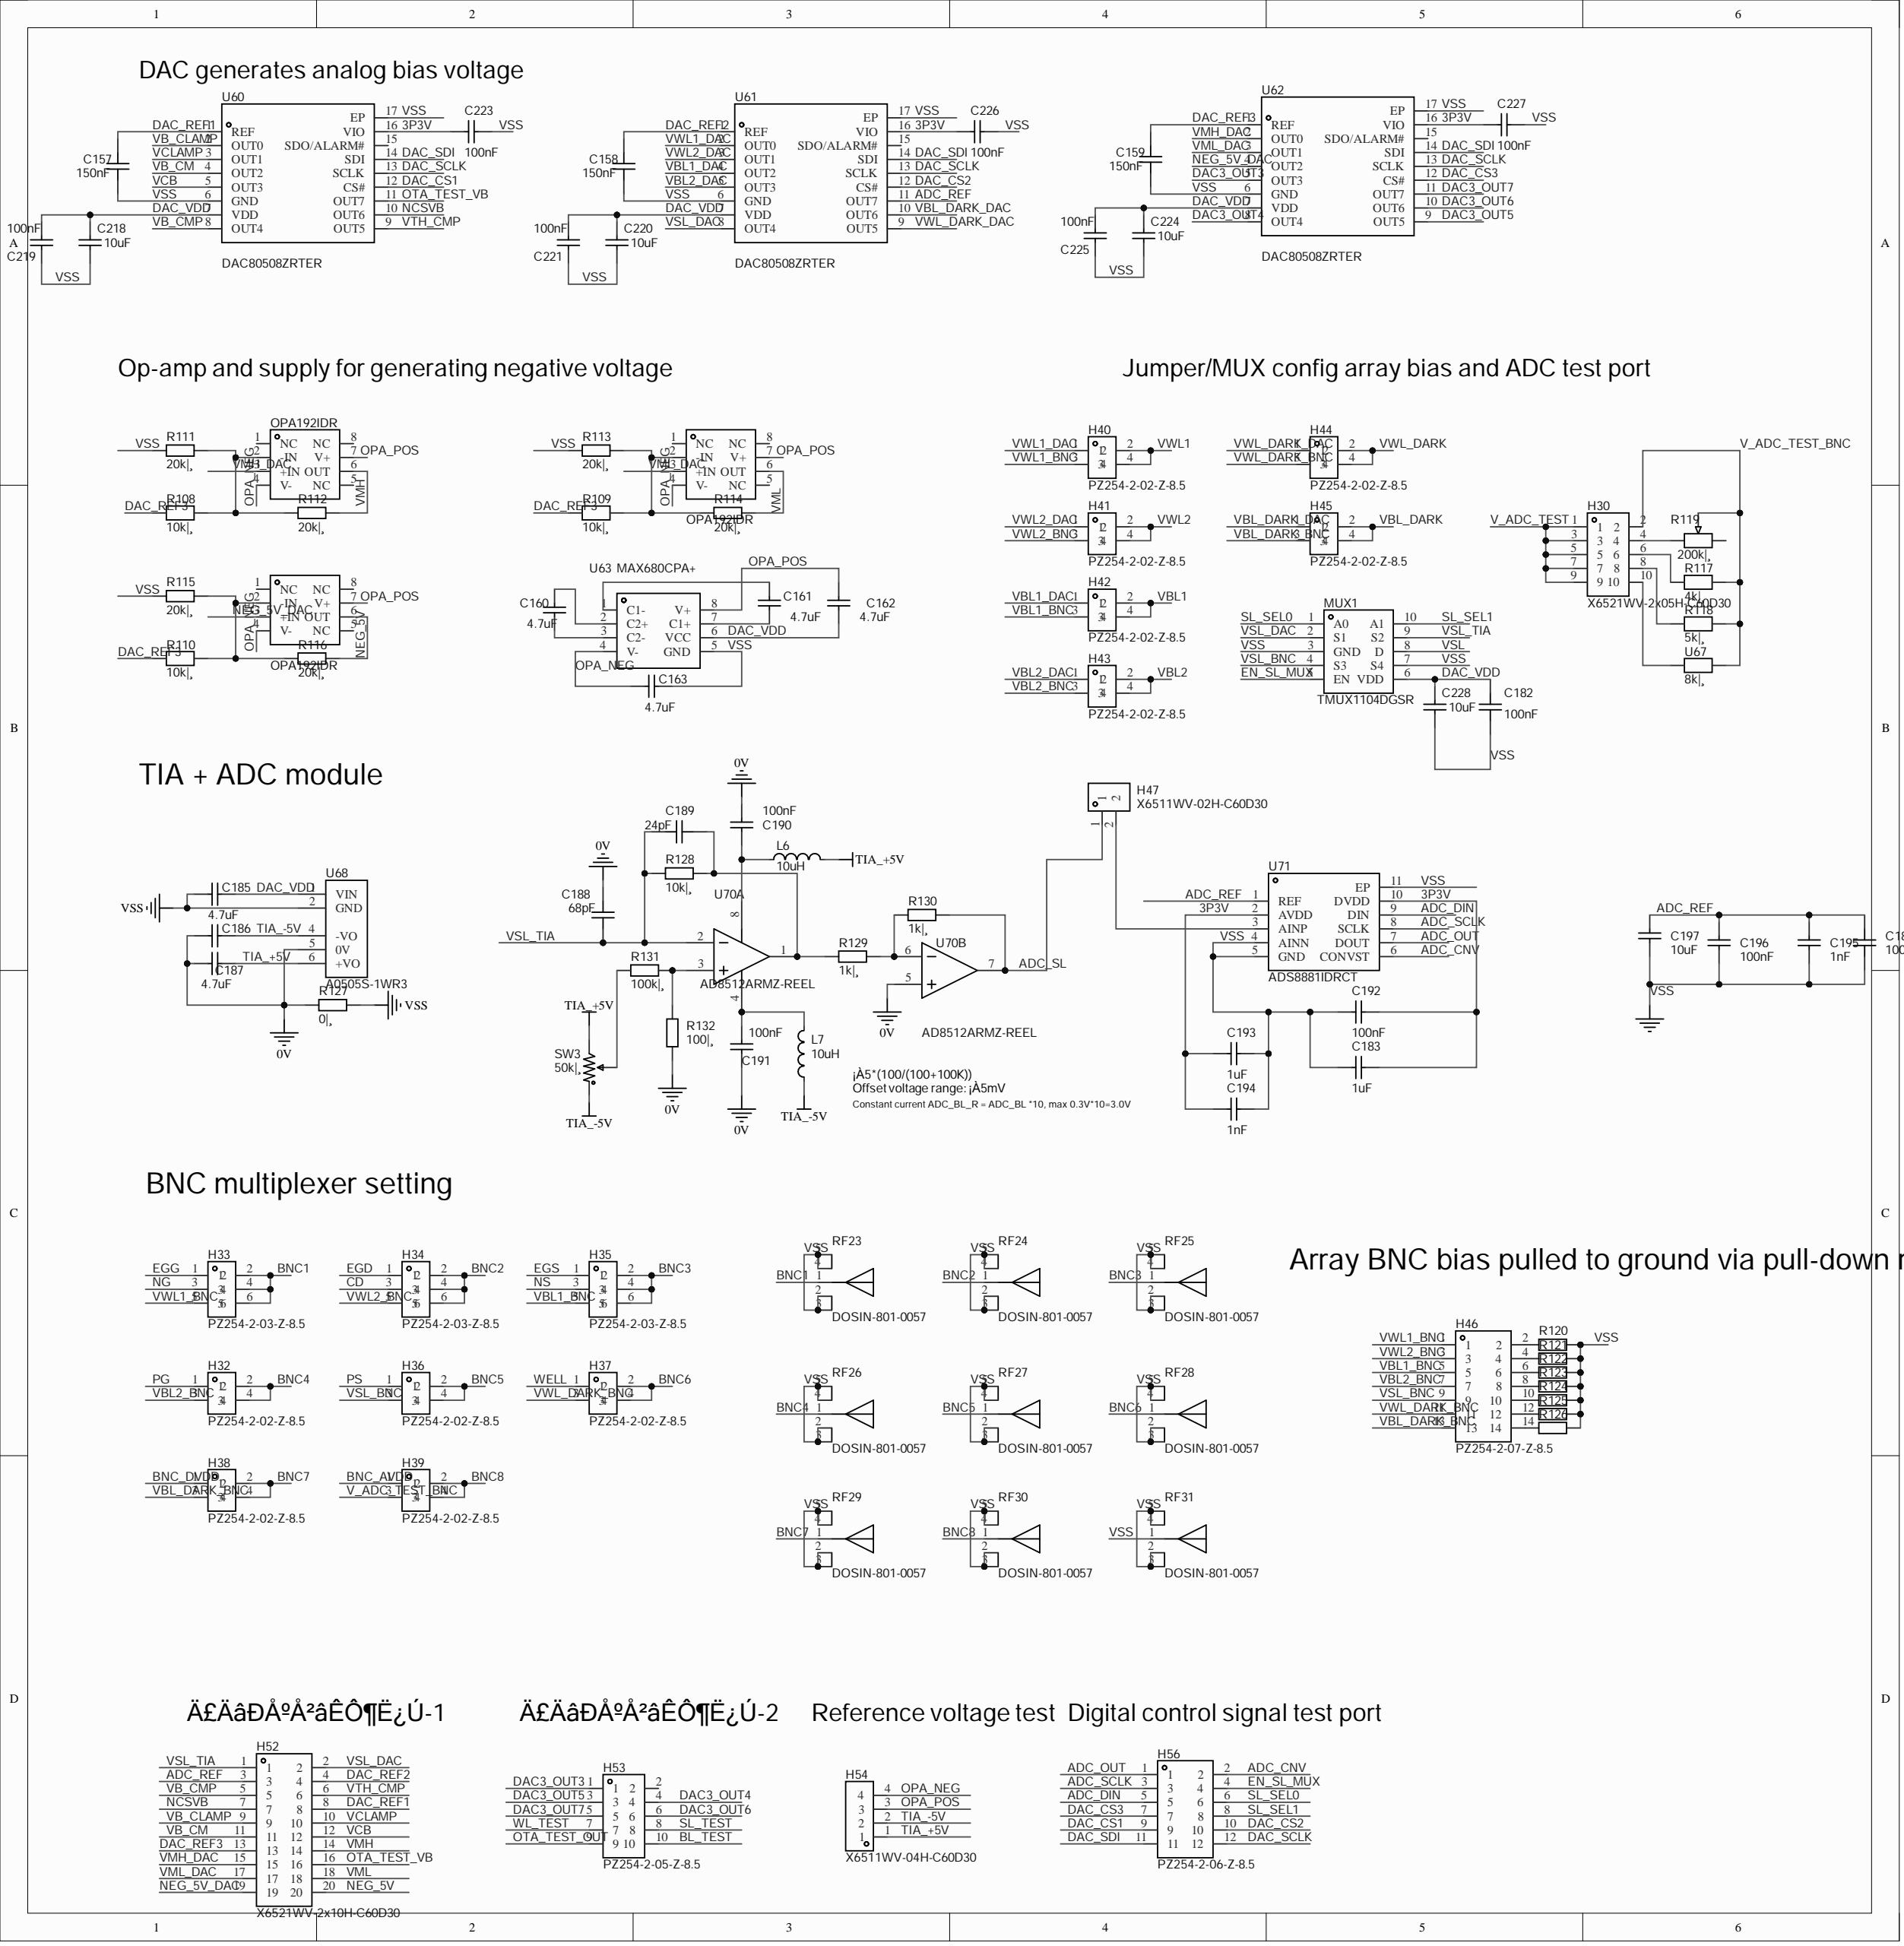Circuit board | Altium Designer | 201 parts | 197 nets | one sheet of the schematic
Parts on this sheet (reference | value | footprint):
C157 | 150nF | C0402
C158 | 150nF | C0402
C159 | 150nF | C0402
C160 | 4.7uF | C0805
C161 | 4.7uF | C0805
C162 | 4.7uF | C0805
C163 | 4.7uF | C0805
C182 | 100nF | C0402
C183 | 1uF | C0603
C184 | 100uF | C1210
C185 | 4.7uF | C0805
C186 | 4.7uF | C0805
C187 | 4.7uF | C0805
C188 | 68pF | C0402
C189 | 24pF | C0402
C190 | 100nF | C0402
C191 | 100nF | C0402
C192 | 100nF | C0402
C193 | 1uF | C0603
C194 | 1nF | C0603
C195 | 1nF | C0603
C196 | 100nF | C0402
C197 | 10uF | C0805
C218 | 10uF | C0805
C219 | 100nF | C0402
C220 | 10uF | C0805
C221 | 100nF | C0402
C223 | 100nF | C0402
C224 | 10uF | C0805
C225 | 100nF | C0402
C226 | 100nF | C0402
C227 | 100nF | C0402
C228 | 10uF | C0805
H30 | X6521WV-2x05H-C60D30 | HDR-TH_10P-P2.54-V-M-R2-C5-S2.54
H32 | PZ254-2-02-Z-8.5 | HDR-TH_4P-P2.54-V-M-R2-C2-S2.54
H33 | PZ254-2-03-Z-8.5 | HDR-TH_6P-P2.54-V-M-R2-C3-S2.54
H34 | PZ254-2-03-Z-8.5 | HDR-TH_6P-P2.54-V-M-R2-C3-S2.54
H35 | PZ254-2-03-Z-8.5 | HDR-TH_6P-P2.54-V-M-R2-C3-S2.54
H36 | PZ254-2-02-Z-8.5 | HDR-TH_4P-P2.54-V-M-R2-C2-S2.54
H37 | PZ254-2-02-Z-8.5 | HDR-TH_4P-P2.54-V-M-R2-C2-S2.54
H38 | PZ254-2-02-Z-8.5 | HDR-TH_4P-P2.54-V-M-R2-C2-S2.54
H39 | PZ254-2-02-Z-8.5 | HDR-TH_4P-P2.54-V-M-R2-C2-S2.54
H40 | PZ254-2-02-Z-8.5 | HDR-TH_4P-P2.54-V-M-R2-C2-S2.54
H41 | PZ254-2-02-Z-8.5 | HDR-TH_4P-P2.54-V-M-R2-C2-S2.54
H42 | PZ254-2-02-Z-8.5 | HDR-TH_4P-P2.54-V-M-R2-C2-S2.54
H43 | PZ254-2-02-Z-8.5 | HDR-TH_4P-P2.54-V-M-R2-C2-S2.54
H44 | PZ254-2-02-Z-8.5 | HDR-TH_4P-P2.54-V-M-R2-C2-S2.54
H45 | PZ254-2-02-Z-8.5 | HDR-TH_4P-P2.54-V-M-R2-C2-S2.54
H46 | PZ254-2-07-Z-8.5 | HDR-TH_14P-P2.54-V-M-R2-C7-S2.54
H47 | X6511WV-02H-C60D30 | HDR-TH_2P-P2.54-V-M
H52 | X6521WV-2x10H-C60D30 | HDR-TH_20P-P2.54-V-M-R2-C10-S2.54
H53 | PZ254-2-05-Z-8.5 | HDR-TH_10P-P2.54-V-M-R2-C5-S2.54
H54 | X6511WV-04H-C60D30 | HDR-TH_4P-P2.54-V-M
H56 | PZ254-2-06-Z-8.5 | HDR-TH_12P-P2.54-V-M-R2-C6-S2.54
L6 | 10uH | IND-SMD_L7.3-W6.8
L7 | 10uH | IND-SMD_L7.3-W6.8
MUX1 | TMUX1104DGSR | VSSOP-10_L3.0-W3.0-P0.50-LS4.9-BL
R108 | 10k|¸ | R0603
R109 | 10k|¸ | R0603
R110 | 10k|¸ | R0603
R111 | 20k|¸ | R0805
R112 | 20k|¸ | R0805
R113 | 20k|¸ | R0805
R114 | 20k|¸ | R0805
R115 | 20k|¸ | R0805
R116 | 20k|¸ | R0805
R117 | 4k|¸ | R0805
R118 | 5k|¸ | R0805
R119 | 200k|¸ | RES-ADJ-SMD_3P-L4.5-W4.5-P2.30-BL-FS
R120 | 1M|¸ | R1206
R121 | 1M|¸ | R1206
R122 | 1M|¸ | R1206
R123 | 1M|¸ | R1206
R124 | 1M|¸ | R1206
R125 | 1M|¸ | R1206
R126 | 1M|¸ | R1206
R127 | 0|¸ | R0603
R128 | 10k|¸ | R0603
R129 | 1k|¸ | R0805
R130 | 1k|¸ | R0805
R131 | 100k|¸ | R0603
R132 | 100|¸ | R1206
RF23 | DOSIN-801-0057 | ANT-TH_DOSIN-801-0057
RF24 | DOSIN-801-0057 | ANT-TH_DOSIN-801-0057
RF25 | DOSIN-801-0057 | ANT-TH_DOSIN-801-0057
RF26 | DOSIN-801-0057 | ANT-TH_DOSIN-801-0057
RF27 | DOSIN-801-0057 | ANT-TH_DOSIN-801-0057
RF28 | DOSIN-801-0057 | ANT-TH_DOSIN-801-0057
RF29 | DOSIN-801-0057 | ANT-TH_DOSIN-801-0057
RF30 | DOSIN-801-0057 | ANT-TH_DOSIN-801-0057
RF31 | DOSIN-801-0057 | ANT-TH_DOSIN-801-0057
SW3 | 50k|¸ | RES-ADJ-SMD_3P-L6.0-W4.3-P5.00-BL
U60 | DAC80508ZRTER | WQFN-16_L3.0-W3.0-P0.50-TL-EP0.8
U61 | DAC80508ZRTER | WQFN-16_L3.0-W3.0-P0.50-TL-EP0.8
U62 | DAC80508ZRTER | WQFN-16_L3.0-W3.0-P0.50-TL-EP0.8
U63 | MAX680CPA+ | DIP-8_L10.1-W6.3-P2.54-LS7.6-BL
U67 | 8k|¸ | R0805
U68 | A0505S-1WR3 | PWRM-TH_A05XXS-1WR3
U71 | ADS8881IDRCT | VSON-10_L3.0-W3.0-P0.50-TL-EP-3
Nets of these parts (net: part-pin ...):
WL_TEST: H53-7
WELL: H37-1
VWL_DARK_DAC: H44-1 U61-9
VWL_DARK_BNC: H37-3 H44-3 H46-11
VWL_DARK: H44-2 H44-4
VWL2_DAC: H41-1 U61-3
VWL2_BNC: H34-5 H41-3 H46-3
VWL2: H41-2 H41-4
VWL1_DAC: H40-1 U61-2
VWL1_BNC: H33-5 H40-3 H46-1
VWL1: H40-2 H40-4
VTH_CMP: H52-6 U60-9
VSS: C157-1 C158-1 C159-1 C163-1 C182-1 C183-1 C184-1 C185-2 C192-2 C193-2 C194-2 C195-1 C196-2 C197-1 C218-1 C219-1 C220-1 C221-1 C223-1 C224-1 C225-1 C226-1 C227-1 C228-1 MUX1-3 MUX1-7 R111-1 R113-1 R115-1 R120-2 R121-2 R122-2 R123-2 R124-2 R125-2 R126-2 R127-2 RF23-2 RF23-3 RF23-4 RF23-5 RF24-2 RF24-3 RF24-4 RF24-5 RF25-2 RF25-3 RF25-4 RF25-5 RF26-2 RF26-3 RF26-4 RF26-5 RF27-2 RF27-3 RF27-4 RF27-5 RF28-2 RF28-3 RF28-4 RF28-5 RF29-2 RF29-3 RF29-4 RF29-5 RF30-2 RF30-3 RF30-4 RF30-5 RF31-1 RF31-2 RF31-3 RF31-4 RF31-5 U60-6 U60-17 U61-6 U61-17 U62-6 U62-17 U63-5 U68-2 U71-4 U71-5 U71-11
VSL_TIA: C188-1 C189-2 H52-1 MUX1-9 R128-1
VSL_DAC: H52-2 MUX1-2 U61-8
VSL_BNC: H36-3 H46-9 MUX1-4
VSL: MUX1-8
VML_DAC: H52-17 U62-3
VML: H52-18 R114-2
VMH_DAC: H52-15 U62-2
VMH: H52-14 R112-2
VCLAMP: H52-10 U60-3
VCB: H52-12 U60-5
VBL_DARK_DAC: H45-1 U61-10
VBL_DARK_BNC: H38-3 H45-3 H46-13
VBL_DARK: H45-2 H45-4
VBL2_DAC: H43-1 U61-5
VBL2_BNC: H32-3 H43-3 H46-7
VBL2: H43-2 H43-4
VBL1_DAC: H42-1 U61-4
VBL1_BNC: H35-5 H42-3 H46-5
VBL1: H42-2 H42-4
VB_CMP: H52-5 U60-8
VB_CM: H52-11 U60-4
VB_CLAMP: H52-9 U60-2
V_ADC_TEST_BNC: H30-2 H39-3 R117-2 R118-2 R119-2 U67-2
V_ADC_TEST: H30-1 H30-3 H30-5 H30-7 H30-9
TIA_-5V: C186-1 H54-2 L7-1 SW3-1 U68-4
TIA_+5V: C187-1 H54-1 L6-2 SW3-3 U68-6
SL_TEST: H53-8
SL_SEL1: H56-8 MUX1-10
SL_SEL0: H56-6 MUX1-1
PS: H36-1
PG: H32-1
OTA_TEST_VB: H52-16 U60-11
OTA_TEST_OUT: H53-9
OPA_POS: C162-2 H54-3 U63-8
OPA_NEG: C163-2 H54-4 U63-4
NS: H35-3
NG: H33-3
NetR131_2: R131-2 R132-2
NetR131_1: R131-1 SW3-2
NetR129_2: R129-2 R130-1
NetR110_2: R110-2 R115-2 R116-1
NetR109_2: R109-2 R113-2 R114-1
NetR108_2: R108-2 R111-2 R112-1
NetH47_2: H47-2 U71-3
NetH46_14: H46-14 R126-1
NetH46_12: H46-12 R125-1
NetH46_10: H46-10 R124-1
NetH46_8: H46-8 R123-1
NetH46_6: H46-6 R122-1
NetH46_4: H46-4 R121-1
NetH46_2: H46-2 R120-1
NetH30_10: H30-10 U67-1
NetH30_8: H30-8 R118-1
NetH30_6: H30-6 R117-1
NetH30_4: H30-4 R119-1
NetC191_2: C191-2 L7-2
NetC190_1: C190-1 L6-1
NetC189_1: C189-1 R128-2 R129-1
NetC161_2: C161-2 U63-1
NetC161_1: C161-1 U63-7
NetC160_2: C160-2 U63-2
NetC160_1: C160-1 U63-3
NEG_5V_DAC: H52-19 U62-4
NEG_5V: H52-20 R116-2
NCSVB: H52-7 U60-10
EN_SL_MUX: H56-4 MUX1-5
EGS: H35-1
EGG: H33-1
EGD: H34-1
DAC_VDD: C162-1 C182-2 C185-1 C218-2 C219-2 C220-2 C221-2 C224-2 C225-2 C228-2 MUX1-6 U60-7 U61-7 U62-7 U63-6 U68-1
DAC_SDI: H56-11 U60-14 U61-14 U62-14
DAC_SCLK: H56-12 U60-13 U61-13 U62-13
DAC_REF3: C159-2 H52-13 R108-1 R109-1 R110-1 U62-1
DAC_REF2: C158-2 H52-4 U61-1
DAC_REF1: C157-2 H52-8 U60-1
DAC_CS3: H56-7 U62-12
DAC_CS2: H56-10 U61-12
DAC_CS1: H56-9 U60-12
DAC3_OUT7: H53-5 U62-11
DAC3_OUT6: H53-6 U62-10
DAC3_OUT5: H53-3 U62-9
DAC3_OUT4: H53-4 U62-8
DAC3_OUT3: H53-1 U62-5
CD: H34-3
BNC_DVDD: H38-1
BNC_AVDD: H39-1
BNC8: H39-2 H39-4 RF30-1
BNC7: H38-2 H38-4 RF29-1
BNC6: H37-2 H37-4 RF28-1
BNC5: H36-2 H36-4 RF27-1
BNC4: H32-2 H32-4 RF26-1
BNC3: H35-2 H35-4 H35-6 RF25-1
BNC2: H34-2 H34-4 H34-6 RF24-1
BNC1: H33-2 H33-4 H33-6 RF23-1
BL_TEST: H53-10
ADC_SL: H47-1 R130-2
ADC_SCLK: H56-3 U71-8
ADC_REF: C184-2 C195-2 C196-1 C197-2 H52-3 U61-11 U71-1
ADC_OUT: H56-1 U71-7
ADC_DIN: H56-5 U71-9
ADC_CNV: H56-2 U71-6
3P3V: C183-2 C192-1 C193-1 C194-1 C223-2 C226-2 C227-2 U60-16 U61-16 U62-16 U71-2 U71-10
0V: C186-2 C187-2 C188-2 C190-2 C191-1 R127-1 R132-1 U68-5